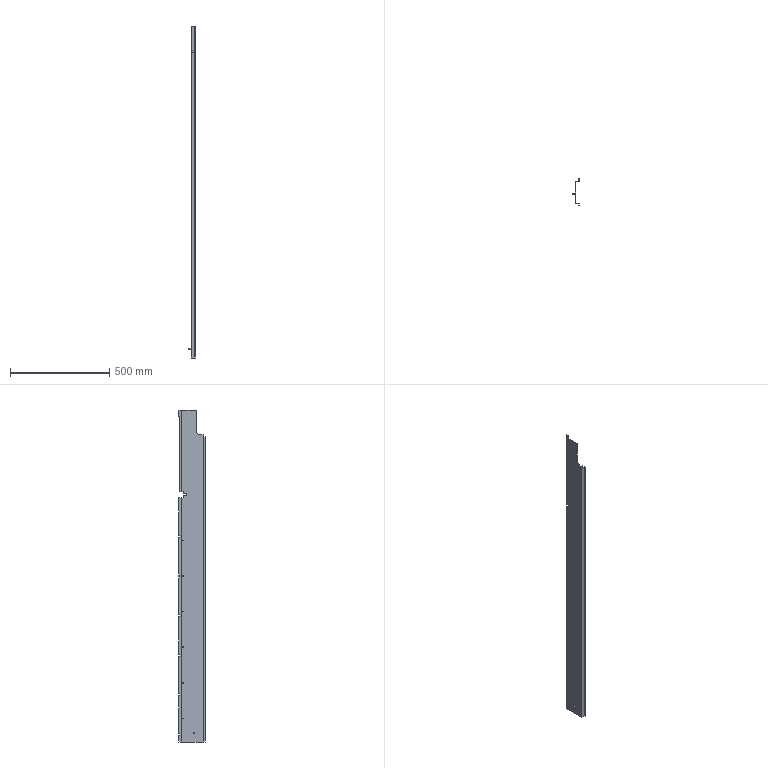Part | STEP file | RJWD-DY-0102_X2_5DE667DC95E8_56 | 1 solid | 106 faces | box 30.5 x 133.9 x 1677 mm | volume 217200 mm3 | plane 74 | cylinder 30 | cone 2 | commonest cylinder face diameters 3.3 x12 0.4 x6 2 x6 6 x4 12 x1 40 x1